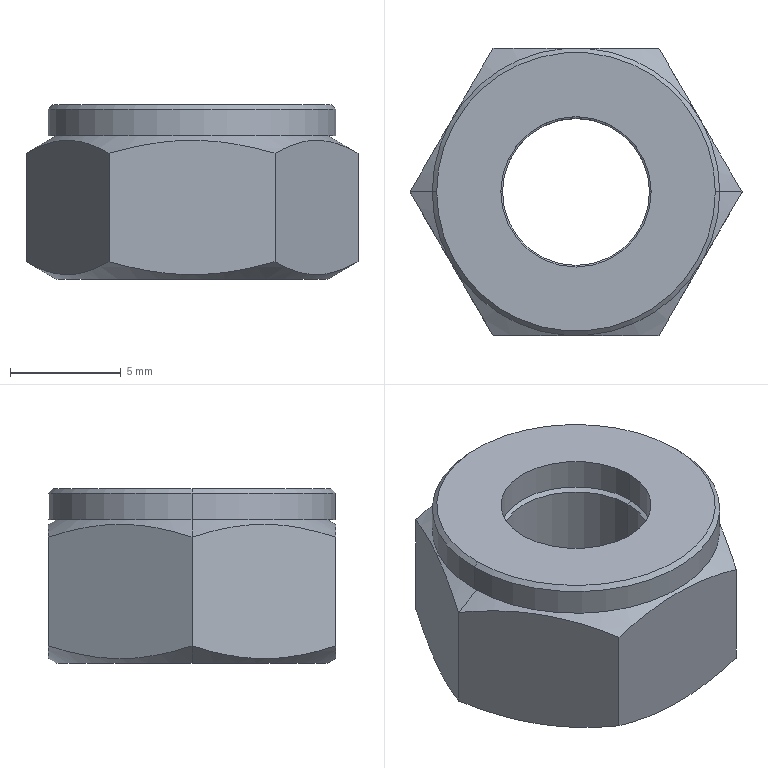Part | SolidWorks | features Chamfer 2, RevCut 2, Extrusion 1, ICE 1, LPattern 1 | 1 solid | 26 faces | box 15.011 x 13 x 7.9 mm | volume 844.03 mm3 | cone 10 | plane 10 | cylinder 6 | commonest cylinder face diameters 6.647 x2 6.8 x2 13 x2
STEP:
#1=CARTESIAN_POINT('',(6.3,0.,1.4));
#2=VERTEX_POINT('',#1);
#3=CARTESIAN_POINT('',(-6.3,0.,1.4));
#4=VERTEX_POINT('',#3);
#5=CARTESIAN_POINT('',(0.,0.,1.4));
#6=DIRECTION('',(0.,0.,1.));
#7=DIRECTION('',(1.,0.,0.));
#8=AXIS2_PLACEMENT_3D('',#5,#6,#7);
#9=CIRCLE('',#8,6.3);
#10=EDGE_CURVE('',#2,#4,#9,.T.);
#11=ORIENTED_EDGE('',*,*,#10,.F.);
#12=CARTESIAN_POINT('',(6.5,0.,1.2));
#13=VERTEX_POINT('',#12);
#14=CARTESIAN_POINT('',(6.3,0.,1.4));
#15=DIRECTION('',(0.7071,0.,-0.7071));
#16=VECTOR('',#15,1000.);
#17=LINE('',#14,#16);
#18=EDGE_CURVE('',#2,#13,#17,.T.);
#19=ORIENTED_EDGE('',*,*,#18,.T.);
#20=CARTESIAN_POINT('',(-6.5,0.,1.2));
#21=VERTEX_POINT('',#20);
#22=CARTESIAN_POINT('',(0.,0.,1.2));
#23=DIRECTION('',(0.,0.,-1.));
#24=DIRECTION('',(1.,0.,0.));
#25=AXIS2_PLACEMENT_3D('',#22,#23,#24);
#26=CIRCLE('',#25,6.5);
#27=EDGE_CURVE('',#21,#13,#26,.T.);
#28=ORIENTED_EDGE('',*,*,#27,.F.);
#29=CARTESIAN_POINT('',(-6.3,0.,1.4));
#30=DIRECTION('',(-0.7071,0.,-0.7071));
#31=VECTOR('',#30,1000.);
#32=LINE('',#29,#31);
#33=EDGE_CURVE('',#4,#21,#32,.T.);
#34=ORIENTED_EDGE('',*,*,#33,.F.);
#35=EDGE_LOOP('',(#11,#19,#28,#34));
#36=FACE_OUTER_BOUND('',#35,.T.);
#37=CARTESIAN_POINT('',(0.,0.,1.4));
#38=DIRECTION('',(0.,0.,-1.));
#39=DIRECTION('',(-1.,0.,0.));
#40=AXIS2_PLACEMENT_3D('',#37,#38,#39);
#41=CONICAL_SURFACE('',#40,6.3,0.7854);
#42=ADVANCED_FACE('',(#36),#41,.T.);
#43=CARTESIAN_POINT('',(-3.4,0.,1.4));
#44=VERTEX_POINT('',#43);
#45=CARTESIAN_POINT('',(3.4,0.,1.4));
#46=VERTEX_POINT('',#45);
#47=CARTESIAN_POINT('',(0.,0.,1.4));
#48=DIRECTION('',(0.,0.,1.));
#49=DIRECTION('',(1.,0.,0.));
#50=AXIS2_PLACEMENT_3D('',#47,#48,#49);
#51=CIRCLE('',#50,3.4);
#52=EDGE_CURVE('',#44,#46,#51,.T.);
#53=ORIENTED_EDGE('',*,*,#52,.T.);
#54=CARTESIAN_POINT('',(3.4,0.,0.));
#55=VERTEX_POINT('',#54);
#56=CARTESIAN_POINT('',(3.4,0.,1.4));
#57=DIRECTION('',(0.,0.,-1.));
#58=VECTOR('',#57,1000.);
#59=LINE('',#56,#58);
#60=EDGE_CURVE('',#46,#55,#59,.T.);
#61=ORIENTED_EDGE('',*,*,#60,.T.);
#62=CARTESIAN_POINT('',(-3.4,0.,0.));
#63=VERTEX_POINT('',#62);
#64=CARTESIAN_POINT('',(0.,0.,0.));
#65=DIRECTION('',(0.,0.,1.));
#66=DIRECTION('',(1.,0.,0.));
#67=AXIS2_PLACEMENT_3D('',#64,#65,#66);
#68=CIRCLE('',#67,3.4);
#69=EDGE_CURVE('',#63,#55,#68,.T.);
#70=ORIENTED_EDGE('',*,*,#69,.F.);
#71=CARTESIAN_POINT('',(-3.4,0.,1.4));
#72=DIRECTION('',(0.,0.,-1.));
#73=VECTOR('',#72,1000.);
#74=LINE('',#71,#73);
#75=EDGE_CURVE('',#44,#63,#74,.T.);
#76=ORIENTED_EDGE('',*,*,#75,.F.);
#77=EDGE_LOOP('',(#53,#61,#70,#76));
#78=FACE_OUTER_BOUND('',#77,.T.);
#79=CARTESIAN_POINT('',(0.,0.,1.4));
#80=DIRECTION('',(0.,0.,-1.));
#81=DIRECTION('',(-1.,0.,0.));
#82=AXIS2_PLACEMENT_3D('',#79,#80,#81);
#83=CYLINDRICAL_SURFACE('',#82,3.4);
#84=ADVANCED_FACE('',(#78),#83,.F.);
#85=ORIENTED_EDGE('',*,*,#27,.T.);
#86=CARTESIAN_POINT('',(6.5,0.,0.));
#87=VERTEX_POINT('',#86);
#88=CARTESIAN_POINT('',(6.5,0.,1.4));
#89=DIRECTION('',(0.,0.,-1.));
#90=VECTOR('',#89,1000.);
#91=LINE('',#88,#90);
#92=EDGE_CURVE('',#13,#87,#91,.T.);
#93=ORIENTED_EDGE('',*,*,#92,.T.);
#94=CARTESIAN_POINT('',(-6.5,0.,0.));
#95=VERTEX_POINT('',#94);
#96=CARTESIAN_POINT('',(0.,0.,0.));
#97=DIRECTION('',(0.,0.,1.));
#98=DIRECTION('',(1.,0.,0.));
#99=AXIS2_PLACEMENT_3D('',#96,#97,#98);
#100=CIRCLE('',#99,6.5);
#101=EDGE_CURVE('',#87,#95,#100,.T.);
#102=ORIENTED_EDGE('',*,*,#101,.T.);
#103=CARTESIAN_POINT('',(-6.5,0.,1.4));
#104=DIRECTION('',(0.,0.,-1.));
#105=VECTOR('',#104,1000.);
#106=LINE('',#103,#105);
#107=EDGE_CURVE('',#21,#95,#106,.T.);
#108=ORIENTED_EDGE('',*,*,#107,.F.);
#109=EDGE_LOOP('',(#85,#93,#102,#108));
#110=FACE_OUTER_BOUND('',#109,.T.);
#111=CARTESIAN_POINT('',(0.,0.,1.4));
#112=DIRECTION('',(0.,0.,-1.));
#113=DIRECTION('',(-1.,0.,0.));
#114=AXIS2_PLACEMENT_3D('',#111,#112,#113);
#115=CYLINDRICAL_SURFACE('',#114,6.5);
#116=ADVANCED_FACE('',(#110),#115,.T.);
#117=CARTESIAN_POINT('',(-3.324,0.,-0.2309));
#118=VERTEX_POINT('',#117);
#119=CARTESIAN_POINT('',(3.323,0.,-0.2309));
#120=VERTEX_POINT('',#119);
#121=CARTESIAN_POINT('',(0.,0.,-0.2309));
#122=DIRECTION('',(0.,0.,1.));
#123=DIRECTION('',(1.,0.,0.));
#124=AXIS2_PLACEMENT_3D('',#121,#122,#123);
#125=CIRCLE('',#124,3.323);
#126=EDGE_CURVE('',#118,#120,#125,.T.);
#127=ORIENTED_EDGE('',*,*,#126,.F.);
#128=CARTESIAN_POINT('',(-3.724,0.,0.));
#129=VERTEX_POINT('',#128);
#130=CARTESIAN_POINT('',(-3.323,0.,-0.2309));
#131=DIRECTION('',(-0.866,0.,0.5));
#132=VECTOR('',#131,1000.);
#133=LINE('',#130,#132);
#134=EDGE_CURVE('',#118,#129,#133,.T.);
#135=ORIENTED_EDGE('',*,*,#134,.T.);
#136=CARTESIAN_POINT('',(3.724,0.,0.));
#137=VERTEX_POINT('',#136);
#138=CARTESIAN_POINT('',(0.,0.,0.));
#139=DIRECTION('',(0.,0.,-1.));
#140=DIRECTION('',(1.,0.,0.));
#141=AXIS2_PLACEMENT_3D('',#138,#139,#140);
#142=CIRCLE('',#141,3.724);
#143=EDGE_CURVE('',#137,#129,#142,.T.);
#144=ORIENTED_EDGE('',*,*,#143,.F.);
#145=CARTESIAN_POINT('',(3.323,0.,-0.2309));
#146=DIRECTION('',(0.866,0.,0.5));
#147=VECTOR('',#146,1000.);
#148=LINE('',#145,#147);
#149=EDGE_CURVE('',#120,#137,#148,.T.);
#150=ORIENTED_EDGE('',*,*,#149,.F.);
#151=EDGE_LOOP('',(#127,#135,#144,#150));
#152=FACE_OUTER_BOUND('',#151,.T.);
#153=CARTESIAN_POINT('',(0.,0.,-0.2309));
#154=DIRECTION('',(0.,0.,1.));
#155=DIRECTION('',(1.,0.,0.));
#156=AXIS2_PLACEMENT_3D('',#153,#154,#155);
#157=CONICAL_SURFACE('',#156,3.323,1.047);
#158=ADVANCED_FACE('',(#152),#157,.F.);
#159=CARTESIAN_POINT('',(3.323,0.,-6.1));
#160=VERTEX_POINT('',#159);
#161=CARTESIAN_POINT('',(-3.324,0.,-6.1));
#162=VERTEX_POINT('',#161);
#163=CARTESIAN_POINT('',(0.,0.,-6.1));
#164=DIRECTION('',(0.,0.,-1.));
#165=DIRECTION('',(1.,0.,0.));
#166=AXIS2_PLACEMENT_3D('',#163,#164,#165);
#167=CIRCLE('',#166,3.323);
#168=EDGE_CURVE('',#160,#162,#167,.T.);
#169=ORIENTED_EDGE('',*,*,#168,.F.);
#170=CARTESIAN_POINT('',(3.554,0.,-6.5));
#171=VERTEX_POINT('',#170);
#172=CARTESIAN_POINT('',(3.554,0.,-6.5));
#173=DIRECTION('',(0.5,0.,-0.866));
#174=VECTOR('',#173,1000.);
#175=LINE('',#172,#174);
#176=EDGE_CURVE('',#160,#171,#175,.T.);
#177=ORIENTED_EDGE('',*,*,#176,.T.);
#178=CARTESIAN_POINT('',(-3.554,0.,-6.5));
#179=VERTEX_POINT('',#178);
#180=CARTESIAN_POINT('',(0.,0.,-6.5));
#181=DIRECTION('',(0.,0.,1.));
#182=DIRECTION('',(1.,0.,0.));
#183=AXIS2_PLACEMENT_3D('',#180,#181,#182);
#184=CIRCLE('',#183,3.554);
#185=EDGE_CURVE('',#179,#171,#184,.T.);
#186=ORIENTED_EDGE('',*,*,#185,.F.);
#187=CARTESIAN_POINT('',(-3.554,0.,-6.5));
#188=DIRECTION('',(-0.5,0.,-0.866));
#189=VECTOR('',#188,1000.);
#190=LINE('',#187,#189);
#191=EDGE_CURVE('',#162,#179,#190,.T.);
#192=ORIENTED_EDGE('',*,*,#191,.F.);
#193=EDGE_LOOP('',(#169,#177,#186,#192));
#194=FACE_OUTER_BOUND('',#193,.T.);
#195=CARTESIAN_POINT('',(0.,0.,-6.5));
#196=DIRECTION('',(0.,0.,-1.));
#197=DIRECTION('',(-1.,0.,0.));
#198=AXIS2_PLACEMENT_3D('',#195,#196,#197);
#199=CONICAL_SURFACE('',#198,3.554,0.5236);
#200=ADVANCED_FACE('',(#194),#199,.F.);
#201=CARTESIAN_POINT('',(-6.125,0.,0.));
#202=VERTEX_POINT('',#201);
#203=CARTESIAN_POINT('',(6.125,0.,0.));
#204=VERTEX_POINT('',#203);
#205=CARTESIAN_POINT('',(0.,0.,0.));
#206=DIRECTION('',(0.,0.,-1.));
#207=DIRECTION('',(-1.,0.,0.));
#208=AXIS2_PLACEMENT_3D('',#205,#206,#207);
#209=CIRCLE('',#208,6.125);
#210=EDGE_CURVE('',#202,#204,#209,.T.);
#211=ORIENTED_EDGE('',*,*,#210,.T.);
#212=CARTESIAN_POINT('',(7.506,0.,-0.7971));
#213=VERTEX_POINT('',#212);
#214=CARTESIAN_POINT('',(6.125,0.,0.));
#215=DIRECTION('',(0.866,0.,-0.5));
#216=VECTOR('',#215,1000.);
#217=LINE('',#214,#216);
#218=EDGE_CURVE('',#204,#213,#217,.T.);
#219=ORIENTED_EDGE('',*,*,#218,.T.);
#220=CARTESIAN_POINT('',(3.753,6.5,-0.7971));
#221=VERTEX_POINT('',#220);
#222=CARTESIAN_POINT('',(7.506,0.,-0.7971));
#223=CARTESIAN_POINT('',(7.199,0.5307,-0.6202));
#224=CARTESIAN_POINT('',(6.891,1.065,-0.4744));
#225=CARTESIAN_POINT('',(6.267,2.145,-0.2724));
#226=CARTESIAN_POINT('',(5.952,2.691,-0.2169));
#227=CARTESIAN_POINT('',(5.473,3.52,-0.2163));
#228=CARTESIAN_POINT('',(5.313,3.798,-0.2299));
#229=CARTESIAN_POINT('',(4.996,4.347,-0.2828));
#230=CARTESIAN_POINT('',(4.838,4.62,-0.3221));
#231=CARTESIAN_POINT('',(4.369,5.433,-0.4738));
#232=CARTESIAN_POINT('',(4.06,5.969,-0.62));
#233=CARTESIAN_POINT('',(3.753,6.5,-0.7971));
#234=B_SPLINE_CURVE_WITH_KNOTS('',3,(#222,#223,#224,#225,#226,#227,#228,#229,#230,#231,#232,#233),.UNSPECIFIED.,.F.,.F.,(4,2,2,2,2,4),(0.000000238,0.001895,0.00379,0.004738,0.005685,0.00758),.UNSPECIFIED.);
#235=EDGE_CURVE('',#213,#221,#234,.T.);
#236=ORIENTED_EDGE('',*,*,#235,.T.);
#237=CARTESIAN_POINT('',(-3.753,6.5,-0.7971));
#238=VERTEX_POINT('',#237);
#239=CARTESIAN_POINT('',(3.753,6.5,-0.7971));
#240=CARTESIAN_POINT('',(3.146,6.5,-0.6219));
#241=CARTESIAN_POINT('',(2.532,6.5,-0.4761));
#242=CARTESIAN_POINT('',(1.278,6.5,-0.2726));
#243=CARTESIAN_POINT('',(0.6353,6.5,-0.2166));
#244=CARTESIAN_POINT('',(-0.6332,6.5,-0.2164));
#245=CARTESIAN_POINT('',(-1.263,6.5,-0.2709));
#246=CARTESIAN_POINT('',(-2.517,6.5,-0.473));
#247=CARTESIAN_POINT('',(-3.142,6.5,-0.6208));
#248=CARTESIAN_POINT('',(-3.753,6.5,-0.7971));
#249=B_SPLINE_CURVE_WITH_KNOTS('',3,(#239,#240,#241,#242,#243,#244,#245,#246,#247,#248),.UNSPECIFIED.,.F.,.F.,(4,2,2,2,4),(0.002787,0.004681,0.006575,0.008469,0.01036),.UNSPECIFIED.);
#250=EDGE_CURVE('',#221,#238,#249,.T.);
#251=ORIENTED_EDGE('',*,*,#250,.T.);
#252=CARTESIAN_POINT('',(-7.506,0.,-0.7971));
#253=VERTEX_POINT('',#252);
#254=CARTESIAN_POINT('',(-3.753,6.5,-0.7971));
#255=CARTESIAN_POINT('',(-4.059,5.969,-0.6202));
#256=CARTESIAN_POINT('',(-4.368,5.435,-0.4744));
#257=CARTESIAN_POINT('',(-4.991,4.355,-0.2724));
#258=CARTESIAN_POINT('',(-5.307,3.809,-0.2169));
#259=CARTESIAN_POINT('',(-5.785,2.98,-0.2163));
#260=CARTESIAN_POINT('',(-5.945,2.702,-0.2299));
#261=CARTESIAN_POINT('',(-6.262,2.153,-0.2828));
#262=CARTESIAN_POINT('',(-6.42,1.88,-0.3221));
#263=CARTESIAN_POINT('',(-6.889,1.067,-0.4738));
#264=CARTESIAN_POINT('',(-7.199,0.5313,-0.62));
#265=CARTESIAN_POINT('',(-7.506,0.,-0.7971));
#266=B_SPLINE_CURVE_WITH_KNOTS('',3,(#254,#255,#256,#257,#258,#259,#260,#261,#262,#263,#264,#265),.UNSPECIFIED.,.F.,.F.,(4,2,2,2,2,4),(0.000000238,0.001895,0.00379,0.004738,0.005685,0.00758),.UNSPECIFIED.);
#267=EDGE_CURVE('',#238,#253,#266,.T.);
#268=ORIENTED_EDGE('',*,*,#267,.T.);
#269=CARTESIAN_POINT('',(-6.125,0.,0.));
#270=DIRECTION('',(-0.866,0.,-0.5));
#271=VECTOR('',#270,1000.);
#272=LINE('',#269,#271);
#273=EDGE_CURVE('',#202,#253,#272,.T.);
#274=ORIENTED_EDGE('',*,*,#273,.F.);
#275=EDGE_LOOP('',(#211,#219,#236,#251,#268,#274));
#276=FACE_OUTER_BOUND('',#275,.T.);
#277=CARTESIAN_POINT('',(0.,0.,0.));
#278=DIRECTION('',(0.,0.,-1.));
#279=DIRECTION('',(-1.,0.,0.));
#280=AXIS2_PLACEMENT_3D('',#277,#278,#279);
#281=CONICAL_SURFACE('',#280,6.125,1.047);
#282=ADVANCED_FACE('',(#276),#281,.T.);
#283=CARTESIAN_POINT('',(-6.125,0.,-6.5));
#284=VERTEX_POINT('',#283);
#285=CARTESIAN_POINT('',(6.125,0.,-6.5));
#286=VERTEX_POINT('',#285);
#287=CARTESIAN_POINT('',(0.,0.,-6.5));
#288=DIRECTION('',(0.,0.,-1.));
#289=DIRECTION('',(-1.,0.,0.));
#290=AXIS2_PLACEMENT_3D('',#287,#288,#289);
#291=CIRCLE('',#290,6.125);
#292=EDGE_CURVE('',#284,#286,#291,.T.);
#293=ORIENTED_EDGE('',*,*,#292,.F.);
#294=CARTESIAN_POINT('',(-7.506,0.,-5.703));
#295=VERTEX_POINT('',#294);
#296=CARTESIAN_POINT('',(-7.506,0.,-5.703));
#297=DIRECTION('',(-0.866,0.,0.5));
#298=VECTOR('',#297,1000.);
#299=LINE('',#296,#298);
#300=EDGE_CURVE('',#284,#295,#299,.T.);
#301=ORIENTED_EDGE('',*,*,#300,.T.);
#302=CARTESIAN_POINT('',(-3.753,6.5,-5.703));
#303=VERTEX_POINT('',#302);
#304=CARTESIAN_POINT('',(-7.506,0.,-5.703));
#305=CARTESIAN_POINT('',(-7.199,0.5307,-5.88));
#306=CARTESIAN_POINT('',(-6.891,1.065,-6.026));
#307=CARTESIAN_POINT('',(-6.267,2.145,-6.228));
#308=CARTESIAN_POINT('',(-5.952,2.691,-6.283));
#309=CARTESIAN_POINT('',(-5.473,3.52,-6.284));
#310=CARTESIAN_POINT('',(-5.313,3.798,-6.27));
#311=CARTESIAN_POINT('',(-4.996,4.347,-6.217));
#312=CARTESIAN_POINT('',(-4.838,4.62,-6.178));
#313=CARTESIAN_POINT('',(-4.369,5.433,-6.026));
#314=CARTESIAN_POINT('',(-4.06,5.969,-5.88));
#315=CARTESIAN_POINT('',(-3.753,6.5,-5.703));
#316=B_SPLINE_CURVE_WITH_KNOTS('',3,(#304,#305,#306,#307,#308,#309,#310,#311,#312,#313,#314,#315),.UNSPECIFIED.,.F.,.F.,(4,2,2,2,2,4),(0.000000238,0.001895,0.00379,0.004738,0.005685,0.00758),.UNSPECIFIED.);
#317=EDGE_CURVE('',#295,#303,#316,.T.);
#318=ORIENTED_EDGE('',*,*,#317,.T.);
#319=CARTESIAN_POINT('',(3.753,6.5,-5.703));
#320=VERTEX_POINT('',#319);
#321=CARTESIAN_POINT('',(-3.753,6.5,-5.703));
#322=CARTESIAN_POINT('',(-3.142,6.5,-5.879));
#323=CARTESIAN_POINT('',(-2.517,6.5,-6.027));
#324=CARTESIAN_POINT('',(-1.263,6.5,-6.229));
#325=CARTESIAN_POINT('',(-0.6332,6.5,-6.284));
#326=CARTESIAN_POINT('',(0.6353,6.5,-6.283));
#327=CARTESIAN_POINT('',(1.278,6.5,-6.227));
#328=CARTESIAN_POINT('',(2.532,6.5,-6.024));
#329=CARTESIAN_POINT('',(3.146,6.5,-5.878));
#330=CARTESIAN_POINT('',(3.753,6.5,-5.703));
#331=B_SPLINE_CURVE_WITH_KNOTS('',3,(#321,#322,#323,#324,#325,#326,#327,#328,#329,#330),.UNSPECIFIED.,.F.,.F.,(4,2,2,2,4),(0.006662,0.008561,0.01046,0.01236,0.01426),.UNSPECIFIED.);
#332=EDGE_CURVE('',#303,#320,#331,.T.);
#333=ORIENTED_EDGE('',*,*,#332,.T.);
#334=CARTESIAN_POINT('',(7.506,0.,-5.703));
#335=VERTEX_POINT('',#334);
#336=CARTESIAN_POINT('',(3.753,6.5,-5.703));
#337=CARTESIAN_POINT('',(4.059,5.969,-5.88));
#338=CARTESIAN_POINT('',(4.368,5.435,-6.026));
#339=CARTESIAN_POINT('',(4.991,4.355,-6.228));
#340=CARTESIAN_POINT('',(5.307,3.809,-6.283));
#341=CARTESIAN_POINT('',(5.785,2.98,-6.284));
#342=CARTESIAN_POINT('',(5.945,2.702,-6.27));
#343=CARTESIAN_POINT('',(6.262,2.153,-6.217));
#344=CARTESIAN_POINT('',(6.42,1.88,-6.178));
#345=CARTESIAN_POINT('',(6.889,1.067,-6.026));
#346=CARTESIAN_POINT('',(7.199,0.5313,-5.88));
#347=CARTESIAN_POINT('',(7.506,0.,-5.703));
#348=B_SPLINE_CURVE_WITH_KNOTS('',3,(#336,#337,#338,#339,#340,#341,#342,#343,#344,#345,#346,#347),.UNSPECIFIED.,.F.,.F.,(4,2,2,2,2,4),(0.000000238,0.001895,0.00379,0.004738,0.005685,0.00758),.UNSPECIFIED.);
#349=EDGE_CURVE('',#320,#335,#348,.T.);
#350=ORIENTED_EDGE('',*,*,#349,.T.);
#351=CARTESIAN_POINT('',(7.506,0.,-5.703));
#352=DIRECTION('',(0.866,0.,0.5));
#353=VECTOR('',#352,1000.);
#354=LINE('',#351,#353);
#355=EDGE_CURVE('',#286,#335,#354,.T.);
#356=ORIENTED_EDGE('',*,*,#355,.F.);
#357=EDGE_LOOP('',(#293,#301,#318,#333,#350,#356));
#358=FACE_OUTER_BOUND('',#357,.T.);
#359=CARTESIAN_POINT('',(0.,0.,-5.703));
#360=DIRECTION('',(0.,0.,1.));
#361=DIRECTION('',(1.,0.,0.));
#362=AXIS2_PLACEMENT_3D('',#359,#360,#361);
#363=CONICAL_SURFACE('',#362,7.506,1.047);
#364=ADVANCED_FACE('',(#358),#363,.T.);
#365=ORIENTED_EDGE('',*,*,#168,.T.);
#366=CARTESIAN_POINT('',(-3.323,0.,-6.5));
#367=DIRECTION('',(0.,0.,1.));
#368=VECTOR('',#367,1000.);
#369=LINE('',#366,#368);
#370=EDGE_CURVE('',#162,#118,#369,.T.);
#371=ORIENTED_EDGE('',*,*,#370,.T.);
#372=ORIENTED_EDGE('',*,*,#126,.T.);
#373=CARTESIAN_POINT('',(3.323,0.,-6.5));
#374=DIRECTION('',(0.,0.,1.));
#375=VECTOR('',#374,1000.);
#376=LINE('',#373,#375);
#377=EDGE_CURVE('',#160,#120,#376,.T.);
#378=ORIENTED_EDGE('',*,*,#377,.F.);
#379=EDGE_LOOP('',(#365,#371,#372,#378));
#380=FACE_OUTER_BOUND('',#379,.T.);
#381=CARTESIAN_POINT('',(0.,0.,-6.5));
#382=DIRECTION('',(0.,0.,1.));
#383=DIRECTION('',(1.,0.,0.));
#384=AXIS2_PLACEMENT_3D('',#381,#382,#383);
#385=CYLINDRICAL_SURFACE('',#384,3.323);
#386=ADVANCED_FACE('',(#380),#385,.F.);
#387=CARTESIAN_POINT('',(-3.753,-6.5,-0.7971));
#388=VERTEX_POINT('',#387);
#389=CARTESIAN_POINT('',(3.753,-6.5,-0.7971));
#390=VERTEX_POINT('',#389);
#391=CARTESIAN_POINT('',(-3.753,-6.5,-0.7971));
#392=CARTESIAN_POINT('',(-3.142,-6.5,-0.6208));
#393=CARTESIAN_POINT('',(-2.517,-6.5,-0.473));
#394=CARTESIAN_POINT('',(-1.263,-6.5,-0.2709));
#395=CARTESIAN_POINT('',(-0.6332,-6.5,-0.2164));
#396=CARTESIAN_POINT('',(0.6353,-6.5,-0.2166));
#397=CARTESIAN_POINT('',(1.278,-6.5,-0.2726));
#398=CARTESIAN_POINT('',(2.532,-6.5,-0.4761));
#399=CARTESIAN_POINT('',(3.146,-6.5,-0.6219));
#400=CARTESIAN_POINT('',(3.753,-6.5,-0.7971));
#401=B_SPLINE_CURVE_WITH_KNOTS('',3,(#391,#392,#393,#394,#395,#396,#397,#398,#399,#400),.UNSPECIFIED.,.F.,.F.,(4,2,2,2,4),(0.006662,0.008561,0.01046,0.01236,0.01426),.UNSPECIFIED.);
#402=EDGE_CURVE('',#388,#390,#401,.T.);
#403=ORIENTED_EDGE('',*,*,#402,.F.);
#404=CARTESIAN_POINT('',(-3.753,-6.5,-5.703));
#405=VERTEX_POINT('',#404);
#406=CARTESIAN_POINT('',(-3.753,-6.5,-6.5));
#407=DIRECTION('',(0.,0.,1.));
#408=VECTOR('',#407,1000.);
#409=LINE('',#406,#408);
#410=EDGE_CURVE('',#405,#388,#409,.T.);
#411=ORIENTED_EDGE('',*,*,#410,.F.);
#412=CARTESIAN_POINT('',(3.753,-6.5,-5.703));
#413=VERTEX_POINT('',#412);
#414=CARTESIAN_POINT('',(3.753,-6.5,-5.703));
#415=CARTESIAN_POINT('',(3.146,-6.5,-5.878));
#416=CARTESIAN_POINT('',(2.532,-6.5,-6.024));
#417=CARTESIAN_POINT('',(1.278,-6.5,-6.227));
#418=CARTESIAN_POINT('',(0.6353,-6.5,-6.283));
#419=CARTESIAN_POINT('',(-0.6332,-6.5,-6.284));
#420=CARTESIAN_POINT('',(-1.263,-6.5,-6.229));
#421=CARTESIAN_POINT('',(-2.517,-6.5,-6.027));
#422=CARTESIAN_POINT('',(-3.142,-6.5,-5.879));
#423=CARTESIAN_POINT('',(-3.753,-6.5,-5.703));
#424=B_SPLINE_CURVE_WITH_KNOTS('',3,(#414,#415,#416,#417,#418,#419,#420,#421,#422,#423),.UNSPECIFIED.,.F.,.F.,(4,2,2,2,4),(0.002787,0.004681,0.006575,0.008469,0.01036),.UNSPECIFIED.);
#425=EDGE_CURVE('',#413,#405,#424,.T.);
#426=ORIENTED_EDGE('',*,*,#425,.F.);
#427=CARTESIAN_POINT('',(3.753,-6.5,-6.5));
#428=DIRECTION('',(0.,0.,1.));
#429=VECTOR('',#428,1000.);
#430=LINE('',#427,#429);
#431=EDGE_CURVE('',#413,#390,#430,.T.);
#432=ORIENTED_EDGE('',*,*,#431,.T.);
#433=EDGE_LOOP('',(#403,#411,#426,#432));
#434=FACE_OUTER_BOUND('',#433,.T.);
#435=CARTESIAN_POINT('',(-3.753,-6.5,-6.5));
#436=DIRECTION('',(0.,-1.,0.));
#437=DIRECTION('',(1.,0.,0.));
#438=AXIS2_PLACEMENT_3D('',#435,#436,#437);
#439=PLANE('',#438);
#440=ADVANCED_FACE('',(#434),#439,.T.);
#441=CARTESIAN_POINT('',(-7.506,0.,-0.7971));
#442=CARTESIAN_POINT('',(-7.199,-0.5307,-0.6202));
#443=CARTESIAN_POINT('',(-6.891,-1.065,-0.4744));
#444=CARTESIAN_POINT('',(-6.267,-2.145,-0.2724));
#445=CARTESIAN_POINT('',(-5.952,-2.691,-0.2169));
#446=CARTESIAN_POINT('',(-5.473,-3.52,-0.2163));
#447=CARTESIAN_POINT('',(-5.313,-3.798,-0.2299));
#448=CARTESIAN_POINT('',(-4.996,-4.347,-0.2828));
#449=CARTESIAN_POINT('',(-4.838,-4.62,-0.3221));
#450=CARTESIAN_POINT('',(-4.369,-5.433,-0.4738));
#451=CARTESIAN_POINT('',(-4.06,-5.969,-0.62));
#452=CARTESIAN_POINT('',(-3.753,-6.5,-0.7971));
#453=B_SPLINE_CURVE_WITH_KNOTS('',3,(#441,#442,#443,#444,#445,#446,#447,#448,#449,#450,#451,#452),.UNSPECIFIED.,.F.,.F.,(4,2,2,2,2,4),(0.000000238,0.001895,0.00379,0.004738,0.005685,0.00758),.UNSPECIFIED.);
#454=EDGE_CURVE('',#253,#388,#453,.T.);
#455=ORIENTED_EDGE('',*,*,#454,.F.);
#456=CARTESIAN_POINT('',(-7.506,0.,-6.5));
#457=DIRECTION('',(0.,0.,1.));
#458=VECTOR('',#457,1000.);
#459=LINE('',#456,#458);
#460=EDGE_CURVE('',#295,#253,#459,.T.);
#461=ORIENTED_EDGE('',*,*,#460,.F.);
#462=CARTESIAN_POINT('',(-3.753,-6.5,-5.703));
#463=CARTESIAN_POINT('',(-4.059,-5.969,-5.88));
#464=CARTESIAN_POINT('',(-4.368,-5.435,-6.026));
#465=CARTESIAN_POINT('',(-4.991,-4.355,-6.228));
#466=CARTESIAN_POINT('',(-5.307,-3.809,-6.283));
#467=CARTESIAN_POINT('',(-5.785,-2.98,-6.284));
#468=CARTESIAN_POINT('',(-5.945,-2.702,-6.27));
#469=CARTESIAN_POINT('',(-6.262,-2.153,-6.217));
#470=CARTESIAN_POINT('',(-6.42,-1.88,-6.178));
#471=CARTESIAN_POINT('',(-6.889,-1.067,-6.026));
#472=CARTESIAN_POINT('',(-7.199,-0.5313,-5.88));
#473=CARTESIAN_POINT('',(-7.506,0.,-5.703));
#474=B_SPLINE_CURVE_WITH_KNOTS('',3,(#462,#463,#464,#465,#466,#467,#468,#469,#470,#471,#472,#473),.UNSPECIFIED.,.F.,.F.,(4,2,2,2,2,4),(0.000000238,0.001895,0.00379,0.004738,0.005685,0.00758),.UNSPECIFIED.);
#475=EDGE_CURVE('',#405,#295,#474,.T.);
#476=ORIENTED_EDGE('',*,*,#475,.F.);
#477=ORIENTED_EDGE('',*,*,#410,.T.);
#478=EDGE_LOOP('',(#455,#461,#476,#477));
#479=FACE_OUTER_BOUND('',#478,.T.);
#480=CARTESIAN_POINT('',(-7.506,0.,-6.5));
#481=DIRECTION('',(-0.866,-0.5,0.));
#482=DIRECTION('',(0.5,-0.866,0.));
#483=AXIS2_PLACEMENT_3D('',#480,#481,#482);
#484=PLANE('',#483);
#485=ADVANCED_FACE('',(#479),#484,.T.);
#486=ORIENTED_EDGE('',*,*,#267,.F.);
#487=CARTESIAN_POINT('',(-3.753,6.5,-6.5));
#488=DIRECTION('',(0.,0.,1.));
#489=VECTOR('',#488,1000.);
#490=LINE('',#487,#489);
#491=EDGE_CURVE('',#303,#238,#490,.T.);
#492=ORIENTED_EDGE('',*,*,#491,.F.);
#493=ORIENTED_EDGE('',*,*,#317,.F.);
#494=ORIENTED_EDGE('',*,*,#460,.T.);
#495=EDGE_LOOP('',(#486,#492,#493,#494));
#496=FACE_OUTER_BOUND('',#495,.T.);
#497=CARTESIAN_POINT('',(-3.753,6.5,-6.5));
#498=DIRECTION('',(-0.866,0.5,0.));
#499=DIRECTION('',(-0.5,-0.866,0.));
#500=AXIS2_PLACEMENT_3D('',#497,#498,#499);
#501=PLANE('',#500);
#502=ADVANCED_FACE('',(#496),#501,.T.);
#503=ORIENTED_EDGE('',*,*,#250,.F.);
#504=CARTESIAN_POINT('',(3.753,6.5,-6.5));
#505=DIRECTION('',(0.,0.,1.));
#506=VECTOR('',#505,1000.);
#507=LINE('',#504,#506);
#508=EDGE_CURVE('',#320,#221,#507,.T.);
#509=ORIENTED_EDGE('',*,*,#508,.F.);
#510=ORIENTED_EDGE('',*,*,#332,.F.);
#511=ORIENTED_EDGE('',*,*,#491,.T.);
#512=EDGE_LOOP('',(#503,#509,#510,#511));
#513=FACE_OUTER_BOUND('',#512,.T.);
#514=CARTESIAN_POINT('',(3.753,6.5,-6.5));
#515=DIRECTION('',(0.,1.,0.));
#516=DIRECTION('',(0.,0.,1.));
#517=AXIS2_PLACEMENT_3D('',#514,#515,#516);
#518=PLANE('',#517);
#519=ADVANCED_FACE('',(#513),#518,.T.);
#520=ORIENTED_EDGE('',*,*,#235,.F.);
#521=CARTESIAN_POINT('',(7.506,0.,-6.5));
#522=DIRECTION('',(0.,0.,1.));
#523=VECTOR('',#522,1000.);
#524=LINE('',#521,#523);
#525=EDGE_CURVE('',#335,#213,#524,.T.);
#526=ORIENTED_EDGE('',*,*,#525,.F.);
#527=ORIENTED_EDGE('',*,*,#349,.F.);
#528=ORIENTED_EDGE('',*,*,#508,.T.);
#529=EDGE_LOOP('',(#520,#526,#527,#528));
#530=FACE_OUTER_BOUND('',#529,.T.);
#531=CARTESIAN_POINT('',(7.506,0.,-6.5));
#532=DIRECTION('',(0.866,0.5,0.));
#533=DIRECTION('',(-0.5,0.866,0.));
#534=AXIS2_PLACEMENT_3D('',#531,#532,#533);
#535=PLANE('',#534);
#536=ADVANCED_FACE('',(#530),#535,.T.);
#537=CARTESIAN_POINT('',(3.753,-6.5,-0.7971));
#538=CARTESIAN_POINT('',(4.059,-5.969,-0.6202));
#539=CARTESIAN_POINT('',(4.368,-5.435,-0.4744));
#540=CARTESIAN_POINT('',(4.991,-4.355,-0.2724));
#541=CARTESIAN_POINT('',(5.307,-3.809,-0.2169));
#542=CARTESIAN_POINT('',(5.785,-2.98,-0.2163));
#543=CARTESIAN_POINT('',(5.945,-2.702,-0.2299));
#544=CARTESIAN_POINT('',(6.262,-2.153,-0.2828));
#545=CARTESIAN_POINT('',(6.42,-1.88,-0.3221));
#546=CARTESIAN_POINT('',(6.889,-1.067,-0.4738));
#547=CARTESIAN_POINT('',(7.199,-0.5313,-0.62));
#548=CARTESIAN_POINT('',(7.506,0.,-0.7971));
#549=B_SPLINE_CURVE_WITH_KNOTS('',3,(#537,#538,#539,#540,#541,#542,#543,#544,#545,#546,#547,#548),.UNSPECIFIED.,.F.,.F.,(4,2,2,2,2,4),(0.000000238,0.001895,0.00379,0.004738,0.005685,0.00758),.UNSPECIFIED.);
#550=EDGE_CURVE('',#390,#213,#549,.T.);
#551=ORIENTED_EDGE('',*,*,#550,.F.);
#552=ORIENTED_EDGE('',*,*,#431,.F.);
#553=CARTESIAN_POINT('',(7.506,0.,-5.703));
#554=CARTESIAN_POINT('',(7.199,-0.5307,-5.88));
#555=CARTESIAN_POINT('',(6.891,-1.065,-6.026));
#556=CARTESIAN_POINT('',(6.267,-2.145,-6.228));
#557=CARTESIAN_POINT('',(5.952,-2.691,-6.283));
#558=CARTESIAN_POINT('',(5.473,-3.52,-6.284));
#559=CARTESIAN_POINT('',(5.313,-3.798,-6.27));
#560=CARTESIAN_POINT('',(4.996,-4.347,-6.217));
#561=CARTESIAN_POINT('',(4.838,-4.62,-6.178));
#562=CARTESIAN_POINT('',(4.369,-5.433,-6.026));
#563=CARTESIAN_POINT('',(4.06,-5.969,-5.88));
#564=CARTESIAN_POINT('',(3.753,-6.5,-5.703));
#565=B_SPLINE_CURVE_WITH_KNOTS('',3,(#553,#554,#555,#556,#557,#558,#559,#560,#561,#562,#563,#564),.UNSPECIFIED.,.F.,.F.,(4,2,2,2,2,4),(0.000000238,0.001895,0.00379,0.004738,0.005685,0.00758),.UNSPECIFIED.);
#566=EDGE_CURVE('',#335,#413,#565,.T.);
#567=ORIENTED_EDGE('',*,*,#566,.F.);
#568=ORIENTED_EDGE('',*,*,#525,.T.);
#569=EDGE_LOOP('',(#551,#552,#567,#568));
#570=FACE_OUTER_BOUND('',#569,.T.);
#571=CARTESIAN_POINT('',(3.753,-6.5,-6.5));
#572=DIRECTION('',(0.866,-0.5,0.));
#573=DIRECTION('',(0.5,0.866,0.));
#574=AXIS2_PLACEMENT_3D('',#571,#572,#573);
#575=PLANE('',#574);
#576=ADVANCED_FACE('',(#570),#575,.T.);
#577=ORIENTED_EDGE('',*,*,#185,.T.);
#578=CARTESIAN_POINT('',(0.,0.,-6.5));
#579=DIRECTION('',(0.,0.,1.));
#580=DIRECTION('',(1.,0.,0.));
#581=AXIS2_PLACEMENT_3D('',#578,#579,#580);
#582=CIRCLE('',#581,3.554);
#583=EDGE_CURVE('',#171,#179,#582,.T.);
#584=ORIENTED_EDGE('',*,*,#583,.T.);
#585=EDGE_LOOP('',(#577,#584));
#586=FACE_BOUND('',#585,.T.);
#587=CARTESIAN_POINT('',(0.,0.,-6.5));
#588=DIRECTION('',(0.,0.,-1.));
#589=DIRECTION('',(-1.,0.,0.));
#590=AXIS2_PLACEMENT_3D('',#587,#588,#589);
#591=CIRCLE('',#590,6.125);
#592=EDGE_CURVE('',#286,#284,#591,.T.);
#593=ORIENTED_EDGE('',*,*,#592,.T.);
#594=ORIENTED_EDGE('',*,*,#292,.T.);
#595=EDGE_LOOP('',(#593,#594));
#596=FACE_OUTER_BOUND('',#595,.T.);
#597=CARTESIAN_POINT('',(3.753,-6.5,-6.5));
#598=DIRECTION('',(0.,0.,1.));
#599=DIRECTION('',(1.,0.,0.));
#600=AXIS2_PLACEMENT_3D('',#597,#598,#599);
#601=PLANE('',#600);
#602=ADVANCED_FACE('',(#586,#596),#601,.F.);
#603=ORIENTED_EDGE('',*,*,#370,.F.);
#604=CARTESIAN_POINT('',(0.,0.,-6.1));
#605=DIRECTION('',(0.,0.,-1.));
#606=DIRECTION('',(1.,0.,0.));
#607=AXIS2_PLACEMENT_3D('',#604,#605,#606);
#608=CIRCLE('',#607,3.323);
#609=EDGE_CURVE('',#162,#160,#608,.T.);
#610=ORIENTED_EDGE('',*,*,#609,.T.);
#611=ORIENTED_EDGE('',*,*,#377,.T.);
#612=CARTESIAN_POINT('',(0.,0.,-0.2309));
#613=DIRECTION('',(0.,0.,1.));
#614=DIRECTION('',(1.,0.,0.));
#615=AXIS2_PLACEMENT_3D('',#612,#613,#614);
#616=CIRCLE('',#615,3.323);
#617=EDGE_CURVE('',#120,#118,#616,.T.);
#618=ORIENTED_EDGE('',*,*,#617,.T.);
#619=EDGE_LOOP('',(#603,#610,#611,#618));
#620=FACE_OUTER_BOUND('',#619,.T.);
#621=CARTESIAN_POINT('',(0.,0.,-6.5));
#622=DIRECTION('',(0.,0.,1.));
#623=DIRECTION('',(1.,0.,0.));
#624=AXIS2_PLACEMENT_3D('',#621,#622,#623);
#625=CYLINDRICAL_SURFACE('',#624,3.323);
#626=ADVANCED_FACE('',(#620),#625,.F.);
#627=ORIENTED_EDGE('',*,*,#300,.F.);
#628=ORIENTED_EDGE('',*,*,#592,.F.);
#629=ORIENTED_EDGE('',*,*,#355,.T.);
#630=ORIENTED_EDGE('',*,*,#566,.T.);
#631=ORIENTED_EDGE('',*,*,#425,.T.);
#632=ORIENTED_EDGE('',*,*,#475,.T.);
#633=EDGE_LOOP('',(#627,#628,#629,#630,#631,#632));
#634=FACE_OUTER_BOUND('',#633,.T.);
#635=CARTESIAN_POINT('',(0.,0.,-5.703));
#636=DIRECTION('',(0.,0.,1.));
#637=DIRECTION('',(1.,0.,0.));
#638=AXIS2_PLACEMENT_3D('',#635,#636,#637);
#639=CONICAL_SURFACE('',#638,7.506,1.047);
#640=ADVANCED_FACE('',(#634),#639,.T.);
#641=ORIENTED_EDGE('',*,*,#218,.F.);
#642=CARTESIAN_POINT('',(0.,0.,0.));
#643=DIRECTION('',(0.,0.,-1.));
#644=DIRECTION('',(-1.,0.,0.));
#645=AXIS2_PLACEMENT_3D('',#642,#643,#644);
#646=CIRCLE('',#645,6.125);
#647=EDGE_CURVE('',#204,#202,#646,.T.);
#648=ORIENTED_EDGE('',*,*,#647,.T.);
#649=ORIENTED_EDGE('',*,*,#273,.T.);
#650=ORIENTED_EDGE('',*,*,#454,.T.);
#651=ORIENTED_EDGE('',*,*,#402,.T.);
#652=ORIENTED_EDGE('',*,*,#550,.T.);
#653=EDGE_LOOP('',(#641,#648,#649,#650,#651,#652));
#654=FACE_OUTER_BOUND('',#653,.T.);
#655=CARTESIAN_POINT('',(0.,0.,0.));
#656=DIRECTION('',(0.,0.,-1.));
#657=DIRECTION('',(-1.,0.,0.));
#658=AXIS2_PLACEMENT_3D('',#655,#656,#657);
#659=CONICAL_SURFACE('',#658,6.125,1.047);
#660=ADVANCED_FACE('',(#654),#659,.T.);
#661=ORIENTED_EDGE('',*,*,#176,.F.);
#662=ORIENTED_EDGE('',*,*,#609,.F.);
#663=ORIENTED_EDGE('',*,*,#191,.T.);
#664=ORIENTED_EDGE('',*,*,#583,.F.);
#665=EDGE_LOOP('',(#661,#662,#663,#664));
#666=FACE_OUTER_BOUND('',#665,.T.);
#667=CARTESIAN_POINT('',(0.,0.,-6.5));
#668=DIRECTION('',(0.,0.,-1.));
#669=DIRECTION('',(-1.,0.,0.));
#670=AXIS2_PLACEMENT_3D('',#667,#668,#669);
#671=CONICAL_SURFACE('',#670,3.554,0.5236);
#672=ADVANCED_FACE('',(#666),#671,.F.);
#673=ORIENTED_EDGE('',*,*,#134,.F.);
#674=ORIENTED_EDGE('',*,*,#617,.F.);
#675=ORIENTED_EDGE('',*,*,#149,.T.);
#676=CARTESIAN_POINT('',(0.,0.,0.));
#677=DIRECTION('',(0.,0.,-1.));
#678=DIRECTION('',(1.,0.,0.));
#679=AXIS2_PLACEMENT_3D('',#676,#677,#678);
#680=CIRCLE('',#679,3.724);
#681=EDGE_CURVE('',#129,#137,#680,.T.);
#682=ORIENTED_EDGE('',*,*,#681,.F.);
#683=EDGE_LOOP('',(#673,#674,#675,#682));
#684=FACE_OUTER_BOUND('',#683,.T.);
#685=CARTESIAN_POINT('',(0.,0.,-0.2309));
#686=DIRECTION('',(0.,0.,1.));
#687=DIRECTION('',(1.,0.,0.));
#688=AXIS2_PLACEMENT_3D('',#685,#686,#687);
#689=CONICAL_SURFACE('',#688,3.323,1.047);
#690=ADVANCED_FACE('',(#684),#689,.F.);
#691=ORIENTED_EDGE('',*,*,#69,.T.);
#692=CARTESIAN_POINT('',(0.,0.,0.));
#693=DIRECTION('',(0.,0.,1.));
#694=DIRECTION('',(1.,0.,0.));
#695=AXIS2_PLACEMENT_3D('',#692,#693,#694);
#696=CIRCLE('',#695,3.4);
#697=EDGE_CURVE('',#55,#63,#696,.T.);
#698=ORIENTED_EDGE('',*,*,#697,.T.);
#699=EDGE_LOOP('',(#691,#698));
#700=FACE_BOUND('',#699,.T.);
#701=ORIENTED_EDGE('',*,*,#143,.T.);
#702=ORIENTED_EDGE('',*,*,#681,.T.);
#703=EDGE_LOOP('',(#701,#702));
#704=FACE_OUTER_BOUND('',#703,.T.);
#705=CARTESIAN_POINT('',(0.,0.,0.));
#706=DIRECTION('',(0.,0.,1.));
#707=DIRECTION('',(1.,0.,0.));
#708=AXIS2_PLACEMENT_3D('',#705,#706,#707);
#709=PLANE('',#708);
#710=ADVANCED_FACE('',(#700,#704),#709,.F.);
#711=CARTESIAN_POINT('',(0.,0.,1.4));
#712=DIRECTION('',(0.,0.,1.));
#713=DIRECTION('',(1.,0.,0.));
#714=AXIS2_PLACEMENT_3D('',#711,#712,#713);
#715=CIRCLE('',#714,6.3);
#716=EDGE_CURVE('',#4,#2,#715,.T.);
#717=ORIENTED_EDGE('',*,*,#716,.T.);
#718=ORIENTED_EDGE('',*,*,#10,.T.);
#719=EDGE_LOOP('',(#717,#718));
#720=FACE_OUTER_BOUND('',#719,.T.);
#721=ORIENTED_EDGE('',*,*,#52,.F.);
#722=CARTESIAN_POINT('',(0.,0.,1.4));
#723=DIRECTION('',(0.,0.,1.));
#724=DIRECTION('',(1.,0.,0.));
#725=AXIS2_PLACEMENT_3D('',#722,#723,#724);
#726=CIRCLE('',#725,3.4);
#727=EDGE_CURVE('',#46,#44,#726,.T.);
#728=ORIENTED_EDGE('',*,*,#727,.F.);
#729=EDGE_LOOP('',(#721,#728));
#730=FACE_BOUND('',#729,.T.);
#731=CARTESIAN_POINT('',(0.,0.,1.4));
#732=DIRECTION('',(0.,0.,1.));
#733=DIRECTION('',(1.,0.,0.));
#734=AXIS2_PLACEMENT_3D('',#731,#732,#733);
#735=PLANE('',#734);
#736=ADVANCED_FACE('',(#720,#730),#735,.T.);
#737=ORIENTED_EDGE('',*,*,#210,.F.);
#738=ORIENTED_EDGE('',*,*,#647,.F.);
#739=EDGE_LOOP('',(#737,#738));
#740=FACE_BOUND('',#739,.T.);
#741=CARTESIAN_POINT('',(0.,0.,0.));
#742=DIRECTION('',(0.,0.,1.));
#743=DIRECTION('',(1.,0.,0.));
#744=AXIS2_PLACEMENT_3D('',#741,#742,#743);
#745=CIRCLE('',#744,6.5);
#746=EDGE_CURVE('',#95,#87,#745,.T.);
#747=ORIENTED_EDGE('',*,*,#746,.F.);
#748=ORIENTED_EDGE('',*,*,#101,.F.);
#749=EDGE_LOOP('',(#747,#748));
#750=FACE_OUTER_BOUND('',#749,.T.);
#751=CARTESIAN_POINT('',(0.,0.,0.));
#752=DIRECTION('',(0.,0.,1.));
#753=DIRECTION('',(1.,0.,0.));
#754=AXIS2_PLACEMENT_3D('',#751,#752,#753);
#755=PLANE('',#754);
#756=ADVANCED_FACE('',(#740,#750),#755,.F.);
#757=ORIENTED_EDGE('',*,*,#92,.F.);
#758=CARTESIAN_POINT('',(0.,0.,1.2));
#759=DIRECTION('',(0.,0.,-1.));
#760=DIRECTION('',(1.,0.,0.));
#761=AXIS2_PLACEMENT_3D('',#758,#759,#760);
#762=CIRCLE('',#761,6.5);
#763=EDGE_CURVE('',#13,#21,#762,.T.);
#764=ORIENTED_EDGE('',*,*,#763,.T.);
#765=ORIENTED_EDGE('',*,*,#107,.T.);
#766=ORIENTED_EDGE('',*,*,#746,.T.);
#767=EDGE_LOOP('',(#757,#764,#765,#766));
#768=FACE_OUTER_BOUND('',#767,.T.);
#769=CARTESIAN_POINT('',(0.,0.,1.4));
#770=DIRECTION('',(0.,0.,-1.));
#771=DIRECTION('',(-1.,0.,0.));
#772=AXIS2_PLACEMENT_3D('',#769,#770,#771);
#773=CYLINDRICAL_SURFACE('',#772,6.5);
#774=ADVANCED_FACE('',(#768),#773,.T.);
#775=ORIENTED_EDGE('',*,*,#60,.F.);
#776=ORIENTED_EDGE('',*,*,#727,.T.);
#777=ORIENTED_EDGE('',*,*,#75,.T.);
#778=ORIENTED_EDGE('',*,*,#697,.F.);
#779=EDGE_LOOP('',(#775,#776,#777,#778));
#780=FACE_OUTER_BOUND('',#779,.T.);
#781=CARTESIAN_POINT('',(0.,0.,1.4));
#782=DIRECTION('',(0.,0.,-1.));
#783=DIRECTION('',(-1.,0.,0.));
#784=AXIS2_PLACEMENT_3D('',#781,#782,#783);
#785=CYLINDRICAL_SURFACE('',#784,3.4);
#786=ADVANCED_FACE('',(#780),#785,.F.);
#787=ORIENTED_EDGE('',*,*,#18,.F.);
#788=ORIENTED_EDGE('',*,*,#716,.F.);
#789=ORIENTED_EDGE('',*,*,#33,.T.);
#790=ORIENTED_EDGE('',*,*,#763,.F.);
#791=EDGE_LOOP('',(#787,#788,#789,#790));
#792=FACE_OUTER_BOUND('',#791,.T.);
#793=CARTESIAN_POINT('',(0.,0.,1.4));
#794=DIRECTION('',(0.,0.,-1.));
#795=DIRECTION('',(-1.,0.,0.));
#796=AXIS2_PLACEMENT_3D('',#793,#794,#795);
#797=CONICAL_SURFACE('',#796,6.3,0.7854);
#798=ADVANCED_FACE('',(#792),#797,.T.);
#799=CLOSED_SHELL('',(#42,#84,#116,#158,#200,#282,#364,#386,#440,#485,#502,#519,#536,#576,#602,#626,#640,#660,#672,#690,#710,#736,#756,#774,#786,#798));
#800=MANIFOLD_SOLID_BREP('',#799);
#801=CARTESIAN_POINT('',(0.,0.,0.));
#802=DIRECTION('',(0.,0.,1.));
#803=DIRECTION('',(1.,0.,0.));
#804=AXIS2_PLACEMENT_3D('',#801,#802,#803);
#805=(LENGTH_UNIT()NAMED_UNIT(*)SI_UNIT(.MILLI.,.METRE.));
#806=UNCERTAINTY_MEASURE_WITH_UNIT(LENGTH_MEASURE(0.00001),#805,'','');
#807=(NAMED_UNIT(*)PLANE_ANGLE_UNIT()SI_UNIT($,.RADIAN.));
#808=(NAMED_UNIT(*)SI_UNIT($,.STERADIAN.)SOLID_ANGLE_UNIT());
#809=(GEOMETRIC_REPRESENTATION_CONTEXT(3)GLOBAL_UNCERTAINTY_ASSIGNED_CONTEXT((#806))GLOBAL_UNIT_ASSIGNED_CONTEXT((#805,#807,#808))REPRESENTATION_CONTEXT('',''));
#810=ADVANCED_BREP_SHAPE_REPRESENTATION('',(#800,#804),#809);